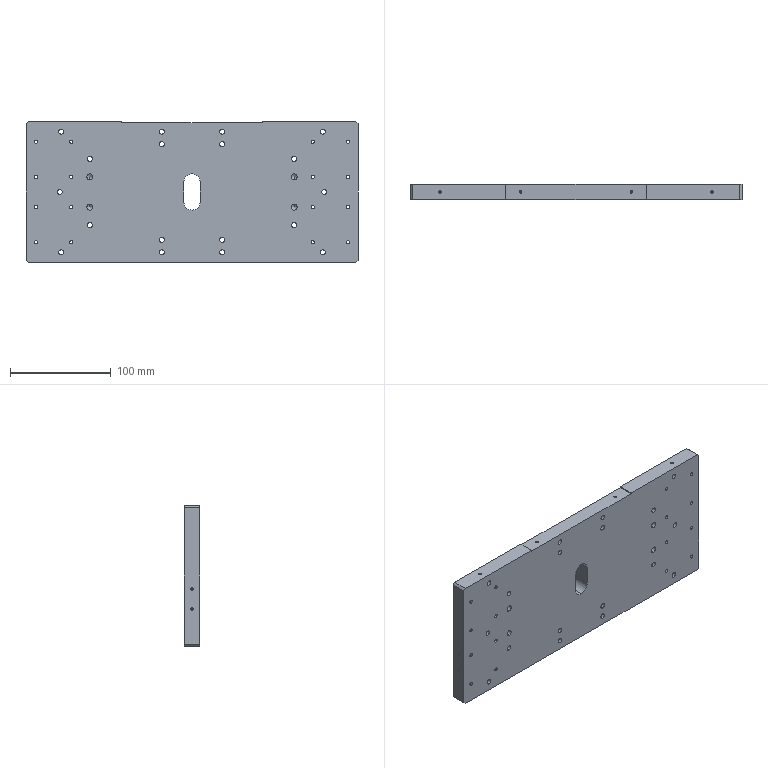Part | SolidWorks | features BaseBody 1 | 1 solid | 151 faces | box 330 x 15 x 140 mm | volume 674027 mm3 | cylinder 103 | cone 32 | plane 16 | commonest cylinder face diameters 5 x36 3.3 x32 2.5 x20 6 x12 16 x3